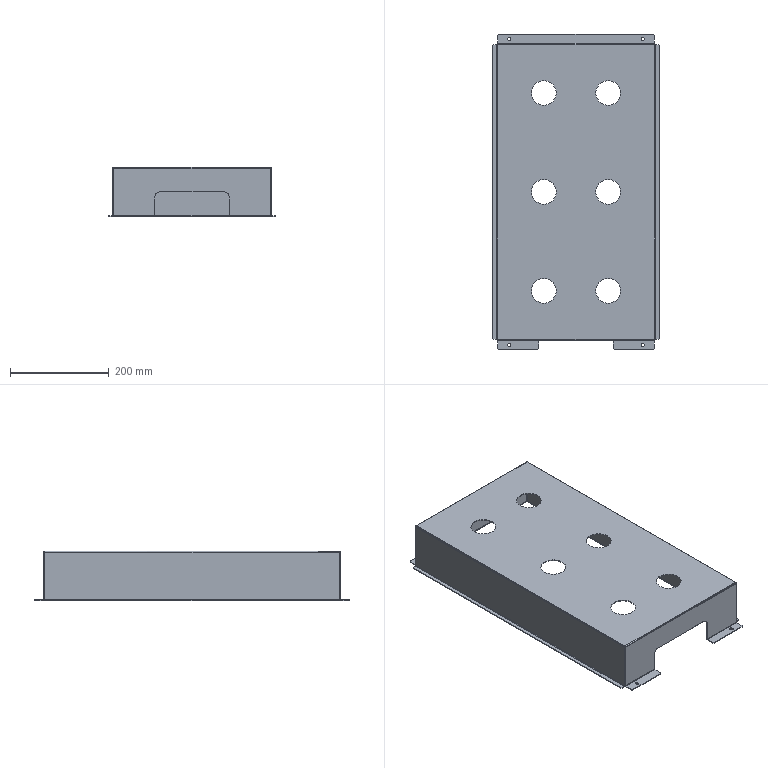Part | SolidWorks | features EdgeFlange 5, ICE 2, Chamfer 1, FlatPattern 1, HoleWzd 1, SMBaseFlange 1, SheetMetal 1 | 1 solid | 122 faces | box 337 x 637 x 100 mm | volume 553796 mm3 | plane 74 | cylinder 40 | spline 8 | commonest cylinder face diameters 50 x12 1.473 x9 4.473 x9 5.5 x8 20 x2